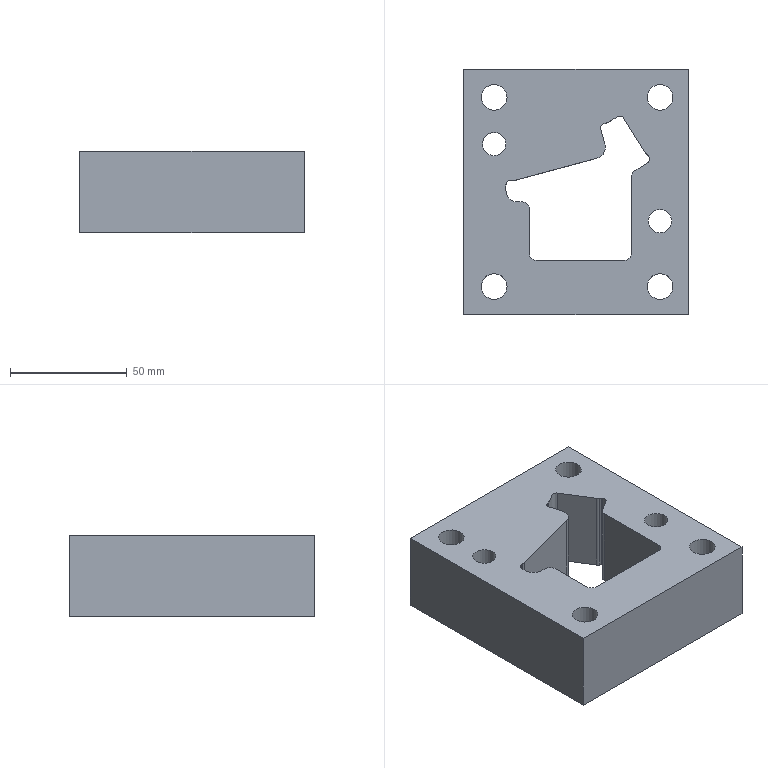Part | NX | features solid 2 | 1 solid | 52 faces | box 96 x 105 x 35 mm | volume 249889 mm3 | cylinder 27 | plane 24 | spline 1 | commonest cylinder face diameters 4 x8 11 x6 10 x5 6 x4 17 x4
STEP:
#1=CARTESIAN_POINT('',(298.719,63.299,43.));
#2=VERTEX_POINT('',#1);
#3=CARTESIAN_POINT('',(298.719,-41.701,43.));
#4=VERTEX_POINT('',#3);
#5=CARTESIAN_POINT('',(298.719,13.399,43.));
#6=DIRECTION('',(0.,-1.,0.));
#7=VECTOR('',#6,1000.);
#8=LINE('',#5,#7);
#9=EDGE_CURVE('',#2,#4,#8,.T.);
#10=ORIENTED_EDGE('',*,*,#9,.T.);
#11=CARTESIAN_POINT('',(298.719,-41.701,78.));
#12=VERTEX_POINT('',#11);
#13=CARTESIAN_POINT('',(298.719,-41.701,-28.));
#14=DIRECTION('',(0.,0.,1.));
#15=VECTOR('',#14,1000.);
#16=LINE('',#13,#15);
#17=EDGE_CURVE('',#4,#12,#16,.T.);
#18=ORIENTED_EDGE('',*,*,#17,.T.);
#19=CARTESIAN_POINT('',(298.719,63.299,78.));
#20=VERTEX_POINT('',#19);
#21=CARTESIAN_POINT('',(298.719,13.399,78.));
#22=DIRECTION('',(0.,-1.,0.));
#23=VECTOR('',#22,1000.);
#24=LINE('',#21,#23);
#25=EDGE_CURVE('',#12,#20,#24,.F.);
#26=ORIENTED_EDGE('',*,*,#25,.T.);
#27=CARTESIAN_POINT('',(298.719,63.299,-28.));
#28=DIRECTION('',(0.,0.,1.));
#29=VECTOR('',#28,1000.);
#30=LINE('',#27,#29);
#31=EDGE_CURVE('',#2,#20,#30,.T.);
#32=ORIENTED_EDGE('',*,*,#31,.F.);
#33=EDGE_LOOP('',(#10,#18,#26,#32));
#34=FACE_BOUND('',#33,.T.);
#35=CARTESIAN_POINT('',(298.719,13.399,-28.));
#36=DIRECTION('',(-1.,0.,0.));
#37=DIRECTION('',(0.,0.,1.));
#38=AXIS2_PLACEMENT_3D('',#35,#36,#37);
#39=PLANE('',#38);
#40=ADVANCED_FACE('',(#34),#39,.T.);
#41=CARTESIAN_POINT('',(394.719,63.299,78.));
#42=VERTEX_POINT('',#41);
#43=CARTESIAN_POINT('',(347.479,63.299,78.));
#44=DIRECTION('',(-1.,0.,0.));
#45=VECTOR('',#44,1000.);
#46=LINE('',#43,#45);
#47=EDGE_CURVE('',#20,#42,#46,.F.);
#48=ORIENTED_EDGE('',*,*,#47,.F.);
#49=ORIENTED_EDGE('',*,*,#25,.F.);
#50=CARTESIAN_POINT('',(394.719,-41.701,78.));
#51=VERTEX_POINT('',#50);
#52=CARTESIAN_POINT('',(347.479,-41.701,78.));
#53=DIRECTION('',(1.,0.,0.));
#54=VECTOR('',#53,1000.);
#55=LINE('',#52,#54);
#56=EDGE_CURVE('',#51,#12,#55,.F.);
#57=ORIENTED_EDGE('',*,*,#56,.F.);
#58=CARTESIAN_POINT('',(394.719,13.399,78.));
#59=DIRECTION('',(0.,1.,0.));
#60=VECTOR('',#59,1000.);
#61=LINE('',#58,#60);
#62=EDGE_CURVE('',#42,#51,#61,.F.);
#63=ORIENTED_EDGE('',*,*,#62,.F.);
#64=EDGE_LOOP('',(#48,#49,#57,#63));
#65=FACE_BOUND('',#64,.T.);
#66=CARTESIAN_POINT('',(387.719,-1.701,78.));
#67=VERTEX_POINT('',#66);
#68=CARTESIAN_POINT('',(382.719,-1.701,78.));
#69=DIRECTION('',(0.,0.,1.));
#70=DIRECTION('',(1.,0.,0.));
#71=AXIS2_PLACEMENT_3D('',#68,#69,#70);
#72=CIRCLE('',#71,5.);
#73=EDGE_CURVE('',#67,#67,#72,.T.);
#74=ORIENTED_EDGE('',*,*,#73,.F.);
#75=EDGE_LOOP('',(#74));
#76=FACE_BOUND('',#75,.T.);
#77=CARTESIAN_POINT('',(316.719,31.299,78.));
#78=VERTEX_POINT('',#77);
#79=CARTESIAN_POINT('',(311.719,31.299,78.));
#80=DIRECTION('',(0.,0.,1.));
#81=DIRECTION('',(1.,0.,0.));
#82=AXIS2_PLACEMENT_3D('',#79,#80,#81);
#83=CIRCLE('',#82,5.);
#84=EDGE_CURVE('',#78,#78,#83,.T.);
#85=ORIENTED_EDGE('',*,*,#84,.F.);
#86=EDGE_LOOP('',(#85));
#87=FACE_BOUND('',#86,.T.);
#88=CARTESIAN_POINT('',(317.219,51.299,78.));
#89=VERTEX_POINT('',#88);
#90=CARTESIAN_POINT('',(311.719,51.299,78.));
#91=DIRECTION('',(0.,0.,-1.));
#92=DIRECTION('',(1.,0.,0.));
#93=AXIS2_PLACEMENT_3D('',#90,#91,#92);
#94=CIRCLE('',#93,5.5);
#95=EDGE_CURVE('',#89,#89,#94,.T.);
#96=ORIENTED_EDGE('',*,*,#95,.T.);
#97=EDGE_LOOP('',(#96));
#98=FACE_BOUND('',#97,.T.);
#99=CARTESIAN_POINT('',(377.219,51.299,78.));
#100=VERTEX_POINT('',#99);
#101=CARTESIAN_POINT('',(382.719,51.299,78.));
#102=DIRECTION('',(0.,0.,1.));
#103=DIRECTION('',(-1.,0.,0.));
#104=AXIS2_PLACEMENT_3D('',#101,#102,#103);
#105=CIRCLE('',#104,5.5);
#106=EDGE_CURVE('',#100,#100,#105,.F.);
#107=ORIENTED_EDGE('',*,*,#106,.T.);
#108=EDGE_LOOP('',(#107));
#109=FACE_BOUND('',#108,.T.);
#110=CARTESIAN_POINT('',(377.219,-29.701,78.));
#111=VERTEX_POINT('',#110);
#112=CARTESIAN_POINT('',(382.719,-29.701,78.));
#113=DIRECTION('',(0.,0.,-1.));
#114=DIRECTION('',(-1.,0.,0.));
#115=AXIS2_PLACEMENT_3D('',#112,#113,#114);
#116=CIRCLE('',#115,5.5);
#117=EDGE_CURVE('',#111,#111,#116,.T.);
#118=ORIENTED_EDGE('',*,*,#117,.T.);
#119=EDGE_LOOP('',(#118));
#120=FACE_BOUND('',#119,.T.);
#121=CARTESIAN_POINT('',(317.219,-29.701,78.));
#122=VERTEX_POINT('',#121);
#123=CARTESIAN_POINT('',(311.719,-29.701,78.));
#124=DIRECTION('',(0.,0.,1.));
#125=DIRECTION('',(1.,0.,0.));
#126=AXIS2_PLACEMENT_3D('',#123,#124,#125);
#127=CIRCLE('',#126,5.5);
#128=EDGE_CURVE('',#122,#122,#127,.T.);
#129=ORIENTED_EDGE('',*,*,#128,.F.);
#130=EDGE_LOOP('',(#129));
#131=FACE_BOUND('',#130,.T.);
#132=CARTESIAN_POINT('',(321.719,6.5,78.));
#133=VERTEX_POINT('',#132);
#134=CARTESIAN_POINT('',(316.719,11.5,78.));
#135=VERTEX_POINT('',#134);
#136=CARTESIAN_POINT('',(321.719,11.5,78.));
#137=DIRECTION('',(0.,0.,-1.));
#138=DIRECTION('',(-1.,0.,0.));
#139=AXIS2_PLACEMENT_3D('',#136,#137,#138);
#140=CIRCLE('',#139,5.);
#141=EDGE_CURVE('',#133,#135,#140,.T.);
#142=ORIENTED_EDGE('',*,*,#141,.T.);
#143=CARTESIAN_POINT('',(316.719,13.767,78.));
#144=VERTEX_POINT('',#143);
#145=CARTESIAN_POINT('',(316.719,89.912,78.));
#146=DIRECTION('',(0.,1.,0.));
#147=VECTOR('',#146,1000.);
#148=LINE('',#145,#147);
#149=EDGE_CURVE('',#135,#144,#148,.T.);
#150=ORIENTED_EDGE('',*,*,#149,.T.);
#151=CARTESIAN_POINT('',(318.201,15.698,78.));
#152=VERTEX_POINT('',#151);
#153=CARTESIAN_POINT('',(318.719,13.767,78.));
#154=DIRECTION('',(0.,0.,-1.));
#155=DIRECTION('',(-1.,0.,0.));
#156=AXIS2_PLACEMENT_3D('',#153,#154,#155);
#157=CIRCLE('',#156,2.);
#158=EDGE_CURVE('',#144,#152,#157,.T.);
#159=ORIENTED_EDGE('',*,*,#158,.T.);
#160=CARTESIAN_POINT('',(318.626,15.812,78.));
#161=VERTEX_POINT('',#160);
#162=CARTESIAN_POINT('',(303.806,11.841,78.));
#163=DIRECTION('',(0.9659,0.2588,0.));
#164=VECTOR('',#163,1000.);
#165=LINE('',#162,#164);
#166=EDGE_CURVE('',#152,#161,#165,.T.);
#167=ORIENTED_EDGE('',*,*,#166,.T.);
#168=CARTESIAN_POINT('',(319.626,15.821,78.));
#169=VERTEX_POINT('',#168);
#170=CARTESIAN_POINT('',(319.143,13.88,78.));
#171=DIRECTION('',(0.,0.,-1.));
#172=DIRECTION('',(-1.,0.,0.));
#173=AXIS2_PLACEMENT_3D('',#170,#171,#172);
#174=CIRCLE('',#173,2.);
#175=EDGE_CURVE('',#161,#169,#174,.T.);
#176=ORIENTED_EDGE('',*,*,#175,.T.);
#177=CARTESIAN_POINT('',(320.626,15.831,78.));
#178=VERTEX_POINT('',#177);
#179=CARTESIAN_POINT('',(320.108,17.762,78.));
#180=DIRECTION('',(0.,0.,-1.));
#181=DIRECTION('',(-1.,0.,0.));
#182=AXIS2_PLACEMENT_3D('',#179,#180,#181);
#183=CIRCLE('',#182,2.);
#184=EDGE_CURVE('',#169,#178,#183,.F.);
#185=ORIENTED_EDGE('',*,*,#184,.T.);
#186=CARTESIAN_POINT('',(355.551,25.189,78.));
#187=VERTEX_POINT('',#186);
#188=CARTESIAN_POINT('',(320.626,15.831,78.));
#189=DIRECTION('',(0.9659,0.2588,0.));
#190=VECTOR('',#189,1000.);
#191=LINE('',#188,#190);
#192=EDGE_CURVE('',#178,#187,#191,.T.);
#193=ORIENTED_EDGE('',*,*,#192,.T.);
#194=CARTESIAN_POINT('',(359.061,31.404,78.));
#195=VERTEX_POINT('',#194);
#196=CARTESIAN_POINT('',(354.257,30.018,78.));
#197=DIRECTION('',(0.,0.,-1.));
#198=DIRECTION('',(-1.,0.,0.));
#199=AXIS2_PLACEMENT_3D('',#196,#197,#198);
#200=CIRCLE('',#199,5.);
#201=EDGE_CURVE('',#187,#195,#200,.F.);
#202=ORIENTED_EDGE('',*,*,#201,.T.);
#203=CARTESIAN_POINT('',(357.296,37.575,78.));
#204=VERTEX_POINT('',#203);
#205=CARTESIAN_POINT('',(359.061,31.404,78.));
#206=CARTESIAN_POINT('',(358.469,33.46,78.));
#207=CARTESIAN_POINT('',(357.879,35.516,78.));
#208=CARTESIAN_POINT('',(357.296,37.575,78.));
#209=B_SPLINE_CURVE_WITH_KNOTS('',3,(#205,#206,#207,#208),.UNSPECIFIED.,.F.,.F.,(4,4),(0.,0.006418),.UNSPECIFIED.);
#210=EDGE_CURVE('',#195,#204,#209,.T.);
#211=ORIENTED_EDGE('',*,*,#210,.T.);
#212=CARTESIAN_POINT('',(358.674,40.044,78.));
#213=VERTEX_POINT('',#212);
#214=CARTESIAN_POINT('',(359.22,38.12,78.));
#215=DIRECTION('',(0.,0.,-1.));
#216=DIRECTION('',(-1.,0.,0.));
#217=AXIS2_PLACEMENT_3D('',#214,#215,#216);
#218=CIRCLE('',#217,2.);
#219=EDGE_CURVE('',#213,#204,#218,.F.);
#220=ORIENTED_EDGE('',*,*,#219,.F.);
#221=CARTESIAN_POINT('',(359.771,40.356,78.));
#222=VERTEX_POINT('',#221);
#223=CARTESIAN_POINT('',(311.762,26.741,78.));
#224=DIRECTION('',(-0.9621,-0.2728,0.));
#225=VECTOR('',#224,1000.);
#226=LINE('',#223,#225);
#227=EDGE_CURVE('',#222,#213,#226,.T.);
#228=ORIENTED_EDGE('',*,*,#227,.F.);
#229=CARTESIAN_POINT('',(361.057,40.926,78.));
#230=VERTEX_POINT('',#229);
#231=CARTESIAN_POINT('',(358.407,45.166,78.));
#232=DIRECTION('',(0.,0.,-1.));
#233=DIRECTION('',(-1.,0.,0.));
#234=AXIS2_PLACEMENT_3D('',#231,#232,#233);
#235=CIRCLE('',#234,5.);
#236=EDGE_CURVE('',#230,#222,#235,.T.);
#237=ORIENTED_EDGE('',*,*,#236,.F.);
#238=CARTESIAN_POINT('',(364.368,42.995,78.));
#239=VERTEX_POINT('',#238);
#240=CARTESIAN_POINT('',(334.735,24.478,78.));
#241=DIRECTION('',(-0.848,-0.5299,0.));
#242=VECTOR('',#241,1000.);
#243=LINE('',#240,#242);
#244=EDGE_CURVE('',#239,#230,#243,.T.);
#245=ORIENTED_EDGE('',*,*,#244,.F.);
#246=CARTESIAN_POINT('',(367.124,42.358,78.));
#247=VERTEX_POINT('',#246);
#248=CARTESIAN_POINT('',(365.428,41.299,78.));
#249=DIRECTION('',(0.,0.,-1.));
#250=DIRECTION('',(-1.,0.,0.));
#251=AXIS2_PLACEMENT_3D('',#248,#249,#250);
#252=CIRCLE('',#251,2.);
#253=EDGE_CURVE('',#247,#239,#252,.F.);
#254=ORIENTED_EDGE('',*,*,#253,.F.);
#255=CARTESIAN_POINT('',(376.282,27.703,78.));
#256=VERTEX_POINT('',#255);
#257=CARTESIAN_POINT('',(367.124,42.358,78.));
#258=DIRECTION('',(0.5299,-0.848,0.));
#259=VECTOR('',#258,1000.);
#260=LINE('',#257,#259);
#261=EDGE_CURVE('',#247,#256,#260,.T.);
#262=ORIENTED_EDGE('',*,*,#261,.T.);
#263=CARTESIAN_POINT('',(377.007,27.014,78.));
#264=VERTEX_POINT('',#263);
#265=CARTESIAN_POINT('',(377.978,28.763,78.));
#266=DIRECTION('',(0.,0.,-1.));
#267=DIRECTION('',(-1.,0.,0.));
#268=AXIS2_PLACEMENT_3D('',#265,#266,#267);
#269=CIRCLE('',#268,2.);
#270=EDGE_CURVE('',#256,#264,#269,.F.);
#271=ORIENTED_EDGE('',*,*,#270,.T.);
#272=CARTESIAN_POINT('',(377.732,26.325,78.));
#273=VERTEX_POINT('',#272);
#274=CARTESIAN_POINT('',(376.036,25.266,78.));
#275=DIRECTION('',(0.,0.,-1.));
#276=DIRECTION('',(-1.,0.,0.));
#277=AXIS2_PLACEMENT_3D('',#274,#275,#276);
#278=CIRCLE('',#277,2.);
#279=EDGE_CURVE('',#264,#273,#278,.T.);
#280=ORIENTED_EDGE('',*,*,#279,.T.);
#281=CARTESIAN_POINT('',(377.937,25.998,78.));
#282=VERTEX_POINT('',#281);
#283=CARTESIAN_POINT('',(375.858,29.324,78.));
#284=DIRECTION('',(0.5299,-0.848,0.));
#285=VECTOR('',#284,1000.);
#286=LINE('',#283,#285);
#287=EDGE_CURVE('',#273,#282,#286,.T.);
#288=ORIENTED_EDGE('',*,*,#287,.T.);
#289=CARTESIAN_POINT('',(377.3,23.242,78.));
#290=VERTEX_POINT('',#289);
#291=CARTESIAN_POINT('',(376.24,24.938,78.));
#292=DIRECTION('',(0.,0.,-1.));
#293=DIRECTION('',(-1.,0.,0.));
#294=AXIS2_PLACEMENT_3D('',#291,#292,#293);
#295=CIRCLE('',#294,2.);
#296=EDGE_CURVE('',#282,#290,#295,.T.);
#297=ORIENTED_EDGE('',*,*,#296,.T.);
#298=CARTESIAN_POINT('',(371.926,19.884,78.));
#299=VERTEX_POINT('',#298);
#300=CARTESIAN_POINT('',(347.244,4.461,78.));
#301=DIRECTION('',(0.848,0.5299,0.));
#302=VECTOR('',#301,1000.);
#303=LINE('',#300,#302);
#304=EDGE_CURVE('',#299,#290,#303,.T.);
#305=ORIENTED_EDGE('',*,*,#304,.F.);
#306=CARTESIAN_POINT('',(370.516,17.34,78.));
#307=VERTEX_POINT('',#306);
#308=CARTESIAN_POINT('',(373.516,17.34,78.));
#309=DIRECTION('',(0.,0.,-1.));
#310=DIRECTION('',(-1.,0.,0.));
#311=AXIS2_PLACEMENT_3D('',#308,#309,#310);
#312=CIRCLE('',#311,3.);
#313=EDGE_CURVE('',#307,#299,#312,.T.);
#314=ORIENTED_EDGE('',*,*,#313,.F.);
#315=CARTESIAN_POINT('',(370.516,-15.5,78.));
#316=VERTEX_POINT('',#315);
#317=CARTESIAN_POINT('',(370.516,0.,78.));
#318=DIRECTION('',(0.,-1.,0.));
#319=VECTOR('',#318,1000.);
#320=LINE('',#317,#319);
#321=EDGE_CURVE('',#316,#307,#320,.F.);
#322=ORIENTED_EDGE('',*,*,#321,.F.);
#323=CARTESIAN_POINT('',(367.516,-18.5,78.));
#324=VERTEX_POINT('',#323);
#325=CARTESIAN_POINT('',(367.516,-15.5,78.));
#326=DIRECTION('',(0.,0.,-1.));
#327=DIRECTION('',(-1.,0.,0.));
#328=AXIS2_PLACEMENT_3D('',#325,#326,#327);
#329=CIRCLE('',#328,3.);
#330=EDGE_CURVE('',#316,#324,#329,.T.);
#331=ORIENTED_EDGE('',*,*,#330,.T.);
#332=CARTESIAN_POINT('',(329.719,-18.5,78.));
#333=VERTEX_POINT('',#332);
#334=CARTESIAN_POINT('',(297.,-18.5,78.));
#335=DIRECTION('',(1.,0.,0.));
#336=VECTOR('',#335,1000.);
#337=LINE('',#334,#336);
#338=EDGE_CURVE('',#333,#324,#337,.T.);
#339=ORIENTED_EDGE('',*,*,#338,.F.);
#340=CARTESIAN_POINT('',(326.719,-15.5,78.));
#341=VERTEX_POINT('',#340);
#342=CARTESIAN_POINT('',(329.719,-15.5,78.));
#343=DIRECTION('',(0.,0.,-1.));
#344=DIRECTION('',(-1.,0.,0.));
#345=AXIS2_PLACEMENT_3D('',#342,#343,#344);
#346=CIRCLE('',#345,3.);
#347=EDGE_CURVE('',#333,#341,#346,.T.);
#348=ORIENTED_EDGE('',*,*,#347,.T.);
#349=CARTESIAN_POINT('',(326.719,3.5,78.));
#350=VERTEX_POINT('',#349);
#351=CARTESIAN_POINT('',(326.719,6.5,78.));
#352=DIRECTION('',(0.,1.,0.));
#353=VECTOR('',#352,1000.);
#354=LINE('',#351,#353);
#355=EDGE_CURVE('',#341,#350,#354,.T.);
#356=ORIENTED_EDGE('',*,*,#355,.T.);
#357=CARTESIAN_POINT('',(323.719,6.5,78.));
#358=VERTEX_POINT('',#357);
#359=CARTESIAN_POINT('',(323.719,3.5,78.));
#360=DIRECTION('',(0.,0.,-1.));
#361=DIRECTION('',(-1.,0.,0.));
#362=AXIS2_PLACEMENT_3D('',#359,#360,#361);
#363=CIRCLE('',#362,3.);
#364=EDGE_CURVE('',#358,#350,#363,.T.);
#365=ORIENTED_EDGE('',*,*,#364,.F.);
#366=CARTESIAN_POINT('',(297.,6.5,78.));
#367=DIRECTION('',(1.,0.,0.));
#368=VECTOR('',#367,1000.);
#369=LINE('',#366,#368);
#370=EDGE_CURVE('',#133,#358,#369,.T.);
#371=ORIENTED_EDGE('',*,*,#370,.F.);
#372=EDGE_LOOP('',(#142,#150,#159,#167,#176,#185,#193,#202,#211,#220,#228,#237,#245,#254,#262,#271,#280,#288,#297,#305,#314,#322,#331,#339,#348,#356,#365,#371));
#373=FACE_BOUND('',#372,.T.);
#374=CARTESIAN_POINT('',(188.,0.,78.));
#375=DIRECTION('',(0.,0.,-1.));
#376=DIRECTION('',(-1.,0.,0.));
#377=AXIS2_PLACEMENT_3D('',#374,#375,#376);
#378=PLANE('',#377);
#379=ADVANCED_FACE('',(#65,#76,#87,#98,#109,#120,#131,#373),#378,.F.);
#380=CARTESIAN_POINT('',(394.719,-41.701,43.));
#381=VERTEX_POINT('',#380);
#382=CARTESIAN_POINT('',(347.479,-41.701,43.));
#383=DIRECTION('',(1.,0.,0.));
#384=VECTOR('',#383,1000.);
#385=LINE('',#382,#384);
#386=EDGE_CURVE('',#4,#381,#385,.T.);
#387=ORIENTED_EDGE('',*,*,#386,.F.);
#388=ORIENTED_EDGE('',*,*,#9,.F.);
#389=CARTESIAN_POINT('',(394.719,63.299,43.));
#390=VERTEX_POINT('',#389);
#391=CARTESIAN_POINT('',(347.479,63.299,43.));
#392=DIRECTION('',(-1.,0.,0.));
#393=VECTOR('',#392,1000.);
#394=LINE('',#391,#393);
#395=EDGE_CURVE('',#390,#2,#394,.T.);
#396=ORIENTED_EDGE('',*,*,#395,.F.);
#397=CARTESIAN_POINT('',(394.719,13.399,43.));
#398=DIRECTION('',(0.,1.,0.));
#399=VECTOR('',#398,1000.);
#400=LINE('',#397,#399);
#401=EDGE_CURVE('',#381,#390,#400,.T.);
#402=ORIENTED_EDGE('',*,*,#401,.F.);
#403=EDGE_LOOP('',(#387,#388,#396,#402));
#404=FACE_BOUND('',#403,.T.);
#405=CARTESIAN_POINT('',(320.219,-29.701,43.));
#406=VERTEX_POINT('',#405);
#407=CARTESIAN_POINT('',(311.719,-29.701,43.));
#408=DIRECTION('',(0.,0.,1.));
#409=DIRECTION('',(1.,0.,0.));
#410=AXIS2_PLACEMENT_3D('',#407,#408,#409);
#411=CIRCLE('',#410,8.5);
#412=EDGE_CURVE('',#406,#406,#411,.T.);
#413=ORIENTED_EDGE('',*,*,#412,.T.);
#414=EDGE_LOOP('',(#413));
#415=FACE_BOUND('',#414,.T.);
#416=CARTESIAN_POINT('',(374.219,-29.701,43.));
#417=VERTEX_POINT('',#416);
#418=CARTESIAN_POINT('',(382.719,-29.701,43.));
#419=DIRECTION('',(0.,0.,-1.));
#420=DIRECTION('',(-1.,0.,0.));
#421=AXIS2_PLACEMENT_3D('',#418,#419,#420);
#422=CIRCLE('',#421,8.5);
#423=EDGE_CURVE('',#417,#417,#422,.F.);
#424=ORIENTED_EDGE('',*,*,#423,.T.);
#425=EDGE_LOOP('',(#424));
#426=FACE_BOUND('',#425,.T.);
#427=CARTESIAN_POINT('',(374.219,51.299,43.));
#428=VERTEX_POINT('',#427);
#429=CARTESIAN_POINT('',(382.719,51.299,43.));
#430=DIRECTION('',(0.,0.,1.));
#431=DIRECTION('',(-1.,0.,0.));
#432=AXIS2_PLACEMENT_3D('',#429,#430,#431);
#433=CIRCLE('',#432,8.5);
#434=EDGE_CURVE('',#428,#428,#433,.T.);
#435=ORIENTED_EDGE('',*,*,#434,.T.);
#436=EDGE_LOOP('',(#435));
#437=FACE_BOUND('',#436,.T.);
#438=CARTESIAN_POINT('',(320.219,51.299,43.));
#439=VERTEX_POINT('',#438);
#440=CARTESIAN_POINT('',(311.719,51.299,43.));
#441=DIRECTION('',(0.,0.,-1.));
#442=DIRECTION('',(1.,0.,0.));
#443=AXIS2_PLACEMENT_3D('',#440,#441,#442);
#444=CIRCLE('',#443,8.5);
#445=EDGE_CURVE('',#439,#439,#444,.F.);
#446=ORIENTED_EDGE('',*,*,#445,.T.);
#447=EDGE_LOOP('',(#446));
#448=FACE_BOUND('',#447,.T.);
#449=CARTESIAN_POINT('',(317.219,31.299,43.));
#450=VERTEX_POINT('',#449);
#451=CARTESIAN_POINT('',(311.719,31.299,43.));
#452=DIRECTION('',(0.,0.,1.));
#453=DIRECTION('',(1.,0.,0.));
#454=AXIS2_PLACEMENT_3D('',#451,#452,#453);
#455=CIRCLE('',#454,5.5);
#456=EDGE_CURVE('',#450,#450,#455,.T.);
#457=ORIENTED_EDGE('',*,*,#456,.T.);
#458=EDGE_LOOP('',(#457));
#459=FACE_BOUND('',#458,.T.);
#460=CARTESIAN_POINT('',(388.219,-1.701,43.));
#461=VERTEX_POINT('',#460);
#462=CARTESIAN_POINT('',(382.719,-1.701,43.));
#463=DIRECTION('',(0.,0.,1.));
#464=DIRECTION('',(1.,0.,0.));
#465=AXIS2_PLACEMENT_3D('',#462,#463,#464);
#466=CIRCLE('',#465,5.5);
#467=EDGE_CURVE('',#461,#461,#466,.T.);
#468=ORIENTED_EDGE('',*,*,#467,.T.);
#469=EDGE_LOOP('',(#468));
#470=FACE_BOUND('',#469,.T.);
#471=CARTESIAN_POINT('',(318.201,15.698,43.));
#472=VERTEX_POINT('',#471);
#473=CARTESIAN_POINT('',(316.719,13.767,43.));
#474=VERTEX_POINT('',#473);
#475=CARTESIAN_POINT('',(318.719,13.767,43.));
#476=DIRECTION('',(0.,0.,-1.));
#477=DIRECTION('',(-1.,0.,0.));
#478=AXIS2_PLACEMENT_3D('',#475,#476,#477);
#479=CIRCLE('',#478,2.);
#480=EDGE_CURVE('',#472,#474,#479,.F.);
#481=ORIENTED_EDGE('',*,*,#480,.T.);
#482=CARTESIAN_POINT('',(316.719,11.5,43.));
#483=VERTEX_POINT('',#482);
#484=CARTESIAN_POINT('',(316.719,0.,43.));
#485=DIRECTION('',(0.,-1.,0.));
#486=VECTOR('',#485,1000.);
#487=LINE('',#484,#486);
#488=EDGE_CURVE('',#474,#483,#487,.T.);
#489=ORIENTED_EDGE('',*,*,#488,.T.);
#490=CARTESIAN_POINT('',(321.719,6.5,43.));
#491=VERTEX_POINT('',#490);
#492=CARTESIAN_POINT('',(321.719,11.5,43.));
#493=DIRECTION('',(0.,0.,-1.));
#494=DIRECTION('',(-1.,0.,0.));
#495=AXIS2_PLACEMENT_3D('',#492,#493,#494);
#496=CIRCLE('',#495,5.);
#497=EDGE_CURVE('',#483,#491,#496,.F.);
#498=ORIENTED_EDGE('',*,*,#497,.T.);
#499=CARTESIAN_POINT('',(323.719,6.5,43.));
#500=VERTEX_POINT('',#499);
#501=CARTESIAN_POINT('',(188.,6.5,43.));
#502=DIRECTION('',(-1.,0.,0.));
#503=VECTOR('',#502,1000.);
#504=LINE('',#501,#503);
#505=EDGE_CURVE('',#500,#491,#504,.T.);
#506=ORIENTED_EDGE('',*,*,#505,.F.);
#507=CARTESIAN_POINT('',(326.719,3.5,43.));
#508=VERTEX_POINT('',#507);
#509=CARTESIAN_POINT('',(323.719,3.5,43.));
#510=DIRECTION('',(0.,0.,-1.));
#511=DIRECTION('',(-1.,0.,0.));
#512=AXIS2_PLACEMENT_3D('',#509,#510,#511);
#513=CIRCLE('',#512,3.);
#514=EDGE_CURVE('',#500,#508,#513,.T.);
#515=ORIENTED_EDGE('',*,*,#514,.T.);
#516=CARTESIAN_POINT('',(326.719,-15.5,43.));
#517=VERTEX_POINT('',#516);
#518=CARTESIAN_POINT('',(326.719,0.,43.));
#519=DIRECTION('',(0.,-1.,0.));
#520=VECTOR('',#519,1000.);
#521=LINE('',#518,#520);
#522=EDGE_CURVE('',#508,#517,#521,.T.);
#523=ORIENTED_EDGE('',*,*,#522,.T.);
#524=CARTESIAN_POINT('',(329.719,-18.5,43.));
#525=VERTEX_POINT('',#524);
#526=CARTESIAN_POINT('',(329.719,-15.5,43.));
#527=DIRECTION('',(0.,0.,-1.));
#528=DIRECTION('',(-1.,0.,0.));
#529=AXIS2_PLACEMENT_3D('',#526,#527,#528);
#530=CIRCLE('',#529,3.);
#531=EDGE_CURVE('',#517,#525,#530,.F.);
#532=ORIENTED_EDGE('',*,*,#531,.T.);
#533=CARTESIAN_POINT('',(367.516,-18.5,43.));
#534=VERTEX_POINT('',#533);
#535=CARTESIAN_POINT('',(188.,-18.5,43.));
#536=DIRECTION('',(-1.,0.,0.));
#537=VECTOR('',#536,1000.);
#538=LINE('',#535,#537);
#539=EDGE_CURVE('',#534,#525,#538,.T.);
#540=ORIENTED_EDGE('',*,*,#539,.F.);
#541=CARTESIAN_POINT('',(370.516,-15.5,43.));
#542=VERTEX_POINT('',#541);
#543=CARTESIAN_POINT('',(367.516,-15.5,43.));
#544=DIRECTION('',(0.,0.,-1.));
#545=DIRECTION('',(-1.,0.,0.));
#546=AXIS2_PLACEMENT_3D('',#543,#544,#545);
#547=CIRCLE('',#546,3.);
#548=EDGE_CURVE('',#534,#542,#547,.F.);
#549=ORIENTED_EDGE('',*,*,#548,.T.);
#550=CARTESIAN_POINT('',(370.516,17.339,43.));
#551=VERTEX_POINT('',#550);
#552=CARTESIAN_POINT('',(370.516,0.,43.));
#553=DIRECTION('',(0.,-1.,0.));
#554=VECTOR('',#553,1000.);
#555=LINE('',#552,#554);
#556=EDGE_CURVE('',#542,#551,#555,.F.);
#557=ORIENTED_EDGE('',*,*,#556,.T.);
#558=CARTESIAN_POINT('',(371.926,19.884,43.));
#559=VERTEX_POINT('',#558);
#560=CARTESIAN_POINT('',(373.516,17.339,43.));
#561=DIRECTION('',(0.,0.,-1.));
#562=DIRECTION('',(-1.,0.,0.));
#563=AXIS2_PLACEMENT_3D('',#560,#561,#562);
#564=CIRCLE('',#563,3.);
#565=EDGE_CURVE('',#551,#559,#564,.T.);
#566=ORIENTED_EDGE('',*,*,#565,.T.);
#567=CARTESIAN_POINT('',(377.3,23.242,43.));
#568=VERTEX_POINT('',#567);
#569=CARTESIAN_POINT('',(230.713,-68.356,43.));
#570=DIRECTION('',(-0.848,-0.5299,0.));
#571=VECTOR('',#570,1000.);
#572=LINE('',#569,#571);
#573=EDGE_CURVE('',#568,#559,#572,.T.);
#574=ORIENTED_EDGE('',*,*,#573,.F.);
#575=CARTESIAN_POINT('',(377.936,25.998,43.));
#576=VERTEX_POINT('',#575);
#577=CARTESIAN_POINT('',(376.24,24.938,43.));
#578=DIRECTION('',(0.,0.,-1.));
#579=DIRECTION('',(-1.,0.,0.));
#580=AXIS2_PLACEMENT_3D('',#577,#578,#579);
#581=CIRCLE('',#580,2.);
#582=EDGE_CURVE('',#568,#576,#581,.F.);
#583=ORIENTED_EDGE('',*,*,#582,.T.);
#584=CARTESIAN_POINT('',(377.732,26.325,43.));
#585=VERTEX_POINT('',#584);
#586=CARTESIAN_POINT('',(336.283,92.657,43.));
#587=DIRECTION('',(-0.5299,0.848,0.));
#588=VECTOR('',#587,1000.);
#589=LINE('',#586,#588);
#590=EDGE_CURVE('',#576,#585,#589,.T.);
#591=ORIENTED_EDGE('',*,*,#590,.T.);
#592=CARTESIAN_POINT('',(377.007,27.014,43.));
#593=VERTEX_POINT('',#592);
#594=CARTESIAN_POINT('',(376.036,25.266,43.));
#595=DIRECTION('',(0.,0.,-1.));
#596=DIRECTION('',(-1.,0.,0.));
#597=AXIS2_PLACEMENT_3D('',#594,#595,#596);
#598=CIRCLE('',#597,2.);
#599=EDGE_CURVE('',#585,#593,#598,.F.);
#600=ORIENTED_EDGE('',*,*,#599,.T.);
#601=CARTESIAN_POINT('',(376.282,27.703,43.));
#602=VERTEX_POINT('',#601);
#603=CARTESIAN_POINT('',(377.978,28.762,43.));
#604=DIRECTION('',(0.,0.,-1.));
#605=DIRECTION('',(-1.,0.,0.));
#606=AXIS2_PLACEMENT_3D('',#603,#604,#605);
#607=CIRCLE('',#606,2.);
#608=EDGE_CURVE('',#593,#602,#607,.T.);
#609=ORIENTED_EDGE('',*,*,#608,.T.);
#610=CARTESIAN_POINT('',(367.124,42.358,43.));
#611=VERTEX_POINT('',#610);
#612=CARTESIAN_POINT('',(335.859,92.392,43.));
#613=DIRECTION('',(-0.5299,0.848,0.));
#614=VECTOR('',#613,1000.);
#615=LINE('',#612,#614);
#616=EDGE_CURVE('',#602,#611,#615,.T.);
#617=ORIENTED_EDGE('',*,*,#616,.T.);
#618=CARTESIAN_POINT('',(364.368,42.995,43.));
#619=VERTEX_POINT('',#618);
#620=CARTESIAN_POINT('',(365.428,41.299,43.));
#621=DIRECTION('',(0.,0.,-1.));
#622=DIRECTION('',(-1.,0.,0.));
#623=AXIS2_PLACEMENT_3D('',#620,#621,#622);
#624=CIRCLE('',#623,2.);
#625=EDGE_CURVE('',#619,#611,#624,.T.);
#626=ORIENTED_EDGE('',*,*,#625,.F.);
#627=CARTESIAN_POINT('',(361.057,40.926,43.));
#628=VERTEX_POINT('',#627);
#629=CARTESIAN_POINT('',(218.205,-48.338,43.));
#630=DIRECTION('',(0.848,0.5299,0.));
#631=VECTOR('',#630,1000.);
#632=LINE('',#629,#631);
#633=EDGE_CURVE('',#628,#619,#632,.T.);
#634=ORIENTED_EDGE('',*,*,#633,.F.);
#635=CARTESIAN_POINT('',(359.771,40.356,43.));
#636=VERTEX_POINT('',#635);
#637=CARTESIAN_POINT('',(358.407,45.166,43.));
#638=DIRECTION('',(0.,0.,-1.));
#639=DIRECTION('',(-1.,0.,0.));
#640=AXIS2_PLACEMENT_3D('',#637,#638,#639);
#641=CIRCLE('',#640,5.);
#642=EDGE_CURVE('',#628,#636,#641,.T.);
#643=ORIENTED_EDGE('',*,*,#642,.T.);
#644=CARTESIAN_POINT('',(358.674,40.044,43.));
#645=VERTEX_POINT('',#644);
#646=CARTESIAN_POINT('',(190.193,-7.734,43.));
#647=DIRECTION('',(0.9621,0.2728,0.));
#648=VECTOR('',#647,1000.);
#649=LINE('',#646,#648);
#650=EDGE_CURVE('',#645,#636,#649,.T.);
#651=ORIENTED_EDGE('',*,*,#650,.F.);
#652=CARTESIAN_POINT('',(357.296,37.575,43.));
#653=VERTEX_POINT('',#652);
#654=CARTESIAN_POINT('',(359.22,38.12,43.));
#655=DIRECTION('',(0.,0.,-1.));
#656=DIRECTION('',(-1.,0.,0.));
#657=AXIS2_PLACEMENT_3D('',#654,#655,#656);
#658=CIRCLE('',#657,2.);
#659=EDGE_CURVE('',#653,#645,#658,.T.);
#660=ORIENTED_EDGE('',*,*,#659,.F.);
#661=CARTESIAN_POINT('',(359.061,31.404,43.));
#662=VERTEX_POINT('',#661);
#663=CARTESIAN_POINT('',(357.296,37.575,43.));
#664=CARTESIAN_POINT('',(357.879,35.516,43.));
#665=CARTESIAN_POINT('',(358.468,33.46,43.));
#666=CARTESIAN_POINT('',(359.061,31.404,43.));
#667=B_SPLINE_CURVE_WITH_KNOTS('',3,(#663,#664,#665,#666),.UNSPECIFIED.,.F.,.F.,(4,4),(0.,0.006418),.UNSPECIFIED.);
#668=EDGE_CURVE('',#653,#662,#667,.T.);
#669=ORIENTED_EDGE('',*,*,#668,.T.);
#670=CARTESIAN_POINT('',(355.551,25.189,43.));
#671=VERTEX_POINT('',#670);
#672=CARTESIAN_POINT('',(354.257,30.018,43.));
#673=DIRECTION('',(0.,0.,-1.));
#674=DIRECTION('',(-1.,0.,0.));
#675=AXIS2_PLACEMENT_3D('',#672,#673,#674);
#676=CIRCLE('',#675,5.);
#677=EDGE_CURVE('',#662,#671,#676,.T.);
#678=ORIENTED_EDGE('',*,*,#677,.T.);
#679=CARTESIAN_POINT('',(320.626,15.831,43.));
#680=VERTEX_POINT('',#679);
#681=CARTESIAN_POINT('',(192.927,-18.386,43.));
#682=DIRECTION('',(-0.9659,-0.2588,0.));
#683=VECTOR('',#682,1000.);
#684=LINE('',#681,#683);
#685=EDGE_CURVE('',#671,#680,#684,.T.);
#686=ORIENTED_EDGE('',*,*,#685,.T.);
#687=CARTESIAN_POINT('',(319.626,15.821,43.));
#688=VERTEX_POINT('',#687);
#689=CARTESIAN_POINT('',(320.108,17.762,43.));
#690=DIRECTION('',(0.,0.,-1.));
#691=DIRECTION('',(-1.,0.,0.));
#692=AXIS2_PLACEMENT_3D('',#689,#690,#691);
#693=CIRCLE('',#692,2.);
#694=EDGE_CURVE('',#680,#688,#693,.T.);
#695=ORIENTED_EDGE('',*,*,#694,.T.);
#696=CARTESIAN_POINT('',(318.626,15.812,43.));
#697=VERTEX_POINT('',#696);
#698=CARTESIAN_POINT('',(319.143,13.88,43.));
#699=DIRECTION('',(0.,0.,-1.));
#700=DIRECTION('',(-1.,0.,0.));
#701=AXIS2_PLACEMENT_3D('',#698,#699,#700);
#702=CIRCLE('',#701,2.);
#703=EDGE_CURVE('',#688,#697,#702,.F.);
#704=ORIENTED_EDGE('',*,*,#703,.T.);
#705=CARTESIAN_POINT('',(192.797,-17.903,43.));
#706=DIRECTION('',(-0.9659,-0.2588,0.));
#707=VECTOR('',#706,1000.);
#708=LINE('',#705,#707);
#709=EDGE_CURVE('',#697,#472,#708,.T.);
#710=ORIENTED_EDGE('',*,*,#709,.T.);
#711=EDGE_LOOP('',(#481,#489,#498,#506,#515,#523,#532,#540,#549,#557,#566,#574,#583,#591,#600,#609,#617,#626,#634,#643,#651,#660,#669,#678,#686,#695,#704,#710));
#712=FACE_BOUND('',#711,.T.);
#713=CARTESIAN_POINT('',(188.,0.,43.));
#714=DIRECTION('',(0.,0.,-1.));
#715=DIRECTION('',(-1.,0.,0.));
#716=AXIS2_PLACEMENT_3D('',#713,#714,#715);
#717=PLANE('',#716);
#718=ADVANCED_FACE('',(#404,#415,#426,#437,#448,#459,#470,#712),#717,.T.);
#719=ORIENTED_EDGE('',*,*,#95,.F.);
#720=EDGE_LOOP('',(#719));
#721=FACE_BOUND('',#720,.T.);
#722=CARTESIAN_POINT('',(317.219,51.299,58.));
#723=VERTEX_POINT('',#722);
#724=CARTESIAN_POINT('',(311.719,51.299,58.));
#725=DIRECTION('',(0.,0.,-1.));
#726=DIRECTION('',(1.,0.,0.));
#727=AXIS2_PLACEMENT_3D('',#724,#725,#726);
#728=CIRCLE('',#727,5.5);
#729=EDGE_CURVE('',#723,#723,#728,.T.);
#730=ORIENTED_EDGE('',*,*,#729,.T.);
#731=EDGE_LOOP('',(#730));
#732=FACE_BOUND('',#731,.T.);
#733=CARTESIAN_POINT('',(311.719,51.299,78.));
#734=DIRECTION('',(0.,0.,1.));
#735=DIRECTION('',(1.,0.,0.));
#736=AXIS2_PLACEMENT_3D('',#733,#734,#735);
#737=CYLINDRICAL_SURFACE('',#736,5.5);
#738=ADVANCED_FACE('',(#721,#732),#737,.F.);
#739=ORIENTED_EDGE('',*,*,#729,.F.);
#740=EDGE_LOOP('',(#739));
#741=FACE_BOUND('',#740,.T.);
#742=CARTESIAN_POINT('',(320.219,51.299,58.));
#743=VERTEX_POINT('',#742);
#744=CARTESIAN_POINT('',(311.719,51.299,58.));
#745=DIRECTION('',(0.,0.,-1.));
#746=DIRECTION('',(1.,0.,0.));
#747=AXIS2_PLACEMENT_3D('',#744,#745,#746);
#748=CIRCLE('',#747,8.5);
#749=EDGE_CURVE('',#743,#743,#748,.T.);
#750=ORIENTED_EDGE('',*,*,#749,.T.);
#751=EDGE_LOOP('',(#750));
#752=FACE_BOUND('',#751,.T.);
#753=CARTESIAN_POINT('',(311.351,49.433,58.));
#754=DIRECTION('',(0.,0.,1.));
#755=DIRECTION('',(1.,0.,0.));
#756=AXIS2_PLACEMENT_3D('',#753,#754,#755);
#757=PLANE('',#756);
#758=ADVANCED_FACE('',(#741,#752),#757,.F.);
#759=ORIENTED_EDGE('',*,*,#749,.F.);
#760=EDGE_LOOP('',(#759));
#761=FACE_BOUND('',#760,.T.);
#762=ORIENTED_EDGE('',*,*,#445,.F.);
#763=EDGE_LOOP('',(#762));
#764=FACE_BOUND('',#763,.T.);
#765=CARTESIAN_POINT('',(311.719,51.299,43.));
#766=DIRECTION('',(0.,0.,1.));
#767=DIRECTION('',(1.,0.,0.));
#768=AXIS2_PLACEMENT_3D('',#765,#766,#767);
#769=CYLINDRICAL_SURFACE('',#768,8.5);
#770=ADVANCED_FACE('',(#761,#764),#769,.F.);
#771=CARTESIAN_POINT('',(374.219,51.299,58.));
#772=VERTEX_POINT('',#771);
#773=CARTESIAN_POINT('',(382.719,51.299,58.));
#774=DIRECTION('',(0.,0.,1.));
#775=DIRECTION('',(-1.,0.,0.));
#776=AXIS2_PLACEMENT_3D('',#773,#774,#775);
#777=CIRCLE('',#776,8.5);
#778=EDGE_CURVE('',#772,#772,#777,.F.);
#779=ORIENTED_EDGE('',*,*,#778,.F.);
#780=EDGE_LOOP('',(#779));
#781=FACE_BOUND('',#780,.T.);
#782=ORIENTED_EDGE('',*,*,#434,.F.);
#783=EDGE_LOOP('',(#782));
#784=FACE_BOUND('',#783,.T.);
#785=CARTESIAN_POINT('',(382.719,51.299,43.));
#786=DIRECTION('',(0.,0.,1.));
#787=DIRECTION('',(-1.,0.,0.));
#788=AXIS2_PLACEMENT_3D('',#785,#786,#787);
#789=CYLINDRICAL_SURFACE('',#788,8.5);
#790=ADVANCED_FACE('',(#781,#784),#789,.F.);
#791=CARTESIAN_POINT('',(377.219,51.299,58.));
#792=VERTEX_POINT('',#791);
#793=CARTESIAN_POINT('',(382.719,51.299,58.));
#794=DIRECTION('',(0.,0.,1.));
#795=DIRECTION('',(-1.,0.,0.));
#796=AXIS2_PLACEMENT_3D('',#793,#794,#795);
#797=CIRCLE('',#796,5.5);
#798=EDGE_CURVE('',#792,#792,#797,.F.);
#799=ORIENTED_EDGE('',*,*,#798,.F.);
#800=EDGE_LOOP('',(#799));
#801=FACE_BOUND('',#800,.T.);
#802=ORIENTED_EDGE('',*,*,#778,.T.);
#803=EDGE_LOOP('',(#802));
#804=FACE_BOUND('',#803,.T.);
#805=CARTESIAN_POINT('',(383.086,49.433,58.));
#806=DIRECTION('',(0.,0.,1.));
#807=DIRECTION('',(-1.,0.,0.));
#808=AXIS2_PLACEMENT_3D('',#805,#806,#807);
#809=PLANE('',#808);
#810=ADVANCED_FACE('',(#801,#804),#809,.F.);
#811=ORIENTED_EDGE('',*,*,#106,.F.);
#812=EDGE_LOOP('',(#811));
#813=FACE_BOUND('',#812,.T.);
#814=ORIENTED_EDGE('',*,*,#798,.T.);
#815=EDGE_LOOP('',(#814));
#816=FACE_BOUND('',#815,.T.);
#817=CARTESIAN_POINT('',(382.719,51.299,78.));
#818=DIRECTION('',(0.,0.,1.));
#819=DIRECTION('',(-1.,0.,0.));
#820=AXIS2_PLACEMENT_3D('',#817,#818,#819);
#821=CYLINDRICAL_SURFACE('',#820,5.5);
#822=ADVANCED_FACE('',(#813,#816),#821,.F.);
#823=CARTESIAN_POINT('',(317.219,-29.701,58.));
#824=VERTEX_POINT('',#823);
#825=CARTESIAN_POINT('',(311.719,-29.701,58.));
#826=DIRECTION('',(0.,0.,1.));
#827=DIRECTION('',(1.,0.,0.));
#828=AXIS2_PLACEMENT_3D('',#825,#826,#827);
#829=CIRCLE('',#828,5.5);
#830=EDGE_CURVE('',#824,#824,#829,.F.);
#831=ORIENTED_EDGE('',*,*,#830,.F.);
#832=EDGE_LOOP('',(#831));
#833=FACE_BOUND('',#832,.T.);
#834=CARTESIAN_POINT('',(320.219,-29.701,58.));
#835=VERTEX_POINT('',#834);
#836=CARTESIAN_POINT('',(311.719,-29.701,58.));
#837=DIRECTION('',(0.,0.,1.));
#838=DIRECTION('',(1.,0.,0.));
#839=AXIS2_PLACEMENT_3D('',#836,#837,#838);
#840=CIRCLE('',#839,8.5);
#841=EDGE_CURVE('',#835,#835,#840,.F.);
#842=ORIENTED_EDGE('',*,*,#841,.T.);
#843=EDGE_LOOP('',(#842));
#844=FACE_BOUND('',#843,.T.);
#845=CARTESIAN_POINT('',(311.351,-27.835,58.));
#846=DIRECTION('',(0.,0.,1.));
#847=DIRECTION('',(1.,0.,0.));
#848=AXIS2_PLACEMENT_3D('',#845,#846,#847);
#849=PLANE('',#848);
#850=ADVANCED_FACE('',(#833,#844),#849,.F.);
#851=CARTESIAN_POINT('',(377.219,-29.701,58.));
#852=VERTEX_POINT('',#851);
#853=CARTESIAN_POINT('',(382.719,-29.701,58.));
#854=DIRECTION('',(0.,0.,-1.));
#855=DIRECTION('',(-1.,0.,0.));
#856=AXIS2_PLACEMENT_3D('',#853,#854,#855);
#857=CIRCLE('',#856,5.5);
#858=EDGE_CURVE('',#852,#852,#857,.T.);
#859=ORIENTED_EDGE('',*,*,#858,.F.);
#860=EDGE_LOOP('',(#859));
#861=FACE_BOUND('',#860,.T.);
#862=CARTESIAN_POINT('',(374.219,-29.701,58.));
#863=VERTEX_POINT('',#862);
#864=CARTESIAN_POINT('',(382.719,-29.701,58.));
#865=DIRECTION('',(0.,0.,-1.));
#866=DIRECTION('',(-1.,0.,0.));
#867=AXIS2_PLACEMENT_3D('',#864,#865,#866);
#868=CIRCLE('',#867,8.5);
#869=EDGE_CURVE('',#863,#863,#868,.T.);
#870=ORIENTED_EDGE('',*,*,#869,.T.);
#871=EDGE_LOOP('',(#870));
#872=FACE_BOUND('',#871,.T.);
#873=CARTESIAN_POINT('',(383.086,-27.835,58.));
#874=DIRECTION('',(0.,0.,1.));
#875=DIRECTION('',(-1.,0.,0.));
#876=AXIS2_PLACEMENT_3D('',#873,#874,#875);
#877=PLANE('',#876);
#878=ADVANCED_FACE('',(#861,#872),#877,.F.);
#879=ORIENTED_EDGE('',*,*,#31,.T.);
#880=ORIENTED_EDGE('',*,*,#47,.T.);
#881=CARTESIAN_POINT('',(394.719,63.299,-28.));
#882=DIRECTION('',(0.,0.,1.));
#883=VECTOR('',#882,1000.);
#884=LINE('',#881,#883);
#885=EDGE_CURVE('',#390,#42,#884,.T.);
#886=ORIENTED_EDGE('',*,*,#885,.F.);
#887=ORIENTED_EDGE('',*,*,#395,.T.);
#888=EDGE_LOOP('',(#879,#880,#886,#887));
#889=FACE_BOUND('',#888,.T.);
#890=CARTESIAN_POINT('',(347.479,63.299,-28.));
#891=DIRECTION('',(0.,1.,0.));
#892=DIRECTION('',(0.,0.,1.));
#893=AXIS2_PLACEMENT_3D('',#890,#891,#892);
#894=PLANE('',#893);
#895=ADVANCED_FACE('',(#889),#894,.T.);
#896=ORIENTED_EDGE('',*,*,#401,.T.);
#897=ORIENTED_EDGE('',*,*,#885,.T.);
#898=ORIENTED_EDGE('',*,*,#62,.T.);
#899=CARTESIAN_POINT('',(394.719,-41.701,-28.));
#900=DIRECTION('',(0.,0.,1.));
#901=VECTOR('',#900,1000.);
#902=LINE('',#899,#901);
#903=EDGE_CURVE('',#381,#51,#902,.T.);
#904=ORIENTED_EDGE('',*,*,#903,.F.);
#905=EDGE_LOOP('',(#896,#897,#898,#904));
#906=FACE_BOUND('',#905,.T.);
#907=CARTESIAN_POINT('',(394.719,13.399,-28.));
#908=DIRECTION('',(1.,0.,0.));
#909=DIRECTION('',(0.,0.,-1.));
#910=AXIS2_PLACEMENT_3D('',#907,#908,#909);
#911=PLANE('',#910);
#912=ADVANCED_FACE('',(#906),#911,.T.);
#913=ORIENTED_EDGE('',*,*,#903,.T.);
#914=ORIENTED_EDGE('',*,*,#56,.T.);
#915=ORIENTED_EDGE('',*,*,#17,.F.);
#916=ORIENTED_EDGE('',*,*,#386,.T.);
#917=EDGE_LOOP('',(#913,#914,#915,#916));
#918=FACE_BOUND('',#917,.T.);
#919=CARTESIAN_POINT('',(347.479,-41.701,-28.));
#920=DIRECTION('',(0.,-1.,0.));
#921=DIRECTION('',(0.,0.,-1.));
#922=AXIS2_PLACEMENT_3D('',#919,#920,#921);
#923=PLANE('',#922);
#924=ADVANCED_FACE('',(#918),#923,.T.);
#925=ORIENTED_EDGE('',*,*,#128,.T.);
#926=EDGE_LOOP('',(#925));
#927=FACE_BOUND('',#926,.T.);
#928=ORIENTED_EDGE('',*,*,#830,.T.);
#929=EDGE_LOOP('',(#928));
#930=FACE_BOUND('',#929,.T.);
#931=CARTESIAN_POINT('',(311.719,-29.701,78.));
#932=DIRECTION('',(0.,0.,1.));
#933=DIRECTION('',(1.,0.,0.));
#934=AXIS2_PLACEMENT_3D('',#931,#932,#933);
#935=CYLINDRICAL_SURFACE('',#934,5.5);
#936=ADVANCED_FACE('',(#927,#930),#935,.F.);
#937=ORIENTED_EDGE('',*,*,#117,.F.);
#938=EDGE_LOOP('',(#937));
#939=FACE_BOUND('',#938,.T.);
#940=ORIENTED_EDGE('',*,*,#858,.T.);
#941=EDGE_LOOP('',(#940));
#942=FACE_BOUND('',#941,.T.);
#943=CARTESIAN_POINT('',(382.719,-29.701,78.));
#944=DIRECTION('',(0.,0.,1.));
#945=DIRECTION('',(-1.,0.,0.));
#946=AXIS2_PLACEMENT_3D('',#943,#944,#945);
#947=CYLINDRICAL_SURFACE('',#946,5.5);
#948=ADVANCED_FACE('',(#939,#942),#947,.F.);
#949=ORIENTED_EDGE('',*,*,#841,.F.);
#950=EDGE_LOOP('',(#949));
#951=FACE_BOUND('',#950,.T.);
#952=ORIENTED_EDGE('',*,*,#412,.F.);
#953=EDGE_LOOP('',(#952));
#954=FACE_BOUND('',#953,.T.);
#955=CARTESIAN_POINT('',(311.719,-29.701,43.));
#956=DIRECTION('',(0.,0.,1.));
#957=DIRECTION('',(1.,0.,0.));
#958=AXIS2_PLACEMENT_3D('',#955,#956,#957);
#959=CYLINDRICAL_SURFACE('',#958,8.5);
#960=ADVANCED_FACE('',(#951,#954),#959,.F.);
#961=ORIENTED_EDGE('',*,*,#869,.F.);
#962=EDGE_LOOP('',(#961));
#963=FACE_BOUND('',#962,.T.);
#964=ORIENTED_EDGE('',*,*,#423,.F.);
#965=EDGE_LOOP('',(#964));
#966=FACE_BOUND('',#965,.T.);
#967=CARTESIAN_POINT('',(382.719,-29.701,43.));
#968=DIRECTION('',(0.,0.,1.));
#969=DIRECTION('',(-1.,0.,0.));
#970=AXIS2_PLACEMENT_3D('',#967,#968,#969);
#971=CYLINDRICAL_SURFACE('',#970,8.5);
#972=ADVANCED_FACE('',(#963,#966),#971,.F.);
#973=ORIENTED_EDGE('',*,*,#84,.T.);
#974=EDGE_LOOP('',(#973));
#975=FACE_BOUND('',#974,.T.);
#976=CARTESIAN_POINT('',(316.719,31.299,58.));
#977=VERTEX_POINT('',#976);
#978=CARTESIAN_POINT('',(311.719,31.299,58.));
#979=DIRECTION('',(0.,0.,1.));
#980=DIRECTION('',(1.,0.,0.));
#981=AXIS2_PLACEMENT_3D('',#978,#979,#980);
#982=CIRCLE('',#981,5.);
#983=EDGE_CURVE('',#977,#977,#982,.F.);
#984=ORIENTED_EDGE('',*,*,#983,.T.);
#985=EDGE_LOOP('',(#984));
#986=FACE_BOUND('',#985,.T.);
#987=CARTESIAN_POINT('',(311.719,31.299,78.));
#988=DIRECTION('',(0.,0.,1.));
#989=DIRECTION('',(1.,0.,0.));
#990=AXIS2_PLACEMENT_3D('',#987,#988,#989);
#991=CYLINDRICAL_SURFACE('',#990,5.);
#992=ADVANCED_FACE('',(#975,#986),#991,.F.);
#993=ORIENTED_EDGE('',*,*,#983,.F.);
#994=EDGE_LOOP('',(#993));
#995=FACE_BOUND('',#994,.T.);
#996=CARTESIAN_POINT('',(317.219,31.299,58.));
#997=VERTEX_POINT('',#996);
#998=CARTESIAN_POINT('',(311.719,31.299,58.));
#999=DIRECTION('',(0.,0.,1.));
#1000=DIRECTION('',(1.,0.,0.));
#1001=AXIS2_PLACEMENT_3D('',#998,#999,#1000);
#1002=CIRCLE('',#1001,5.5);
#1003=EDGE_CURVE('',#997,#997,#1002,.F.);
#1004=ORIENTED_EDGE('',*,*,#1003,.T.);
#1005=EDGE_LOOP('',(#1004));
#1006=FACE_BOUND('',#1005,.T.);
#1007=CARTESIAN_POINT('',(312.444,30.227,58.));
#1008=DIRECTION('',(0.,0.,1.));
#1009=DIRECTION('',(1.,0.,0.));
#1010=AXIS2_PLACEMENT_3D('',#1007,#1008,#1009);
#1011=PLANE('',#1010);
#1012=ADVANCED_FACE('',(#995,#1006),#1011,.F.);
#1013=ORIENTED_EDGE('',*,*,#1003,.F.);
#1014=EDGE_LOOP('',(#1013));
#1015=FACE_BOUND('',#1014,.T.);
#1016=ORIENTED_EDGE('',*,*,#456,.F.);
#1017=EDGE_LOOP('',(#1016));
#1018=FACE_BOUND('',#1017,.T.);
#1019=CARTESIAN_POINT('',(311.719,31.299,43.));
#1020=DIRECTION('',(0.,0.,1.));
#1021=DIRECTION('',(1.,0.,0.));
#1022=AXIS2_PLACEMENT_3D('',#1019,#1020,#1021);
#1023=CYLINDRICAL_SURFACE('',#1022,5.5);
#1024=ADVANCED_FACE('',(#1015,#1018),#1023,.F.);
#1025=ORIENTED_EDGE('',*,*,#73,.T.);
#1026=EDGE_LOOP('',(#1025));
#1027=FACE_BOUND('',#1026,.T.);
#1028=CARTESIAN_POINT('',(387.719,-1.701,58.));
#1029=VERTEX_POINT('',#1028);
#1030=CARTESIAN_POINT('',(382.719,-1.701,58.));
#1031=DIRECTION('',(0.,0.,1.));
#1032=DIRECTION('',(1.,0.,0.));
#1033=AXIS2_PLACEMENT_3D('',#1030,#1031,#1032);
#1034=CIRCLE('',#1033,5.);
#1035=EDGE_CURVE('',#1029,#1029,#1034,.F.);
#1036=ORIENTED_EDGE('',*,*,#1035,.T.);
#1037=EDGE_LOOP('',(#1036));
#1038=FACE_BOUND('',#1037,.T.);
#1039=CARTESIAN_POINT('',(382.719,-1.701,78.));
#1040=DIRECTION('',(0.,0.,1.));
#1041=DIRECTION('',(1.,0.,0.));
#1042=AXIS2_PLACEMENT_3D('',#1039,#1040,#1041);
#1043=CYLINDRICAL_SURFACE('',#1042,5.);
#1044=ADVANCED_FACE('',(#1027,#1038),#1043,.F.);
#1045=ORIENTED_EDGE('',*,*,#1035,.F.);
#1046=EDGE_LOOP('',(#1045));
#1047=FACE_BOUND('',#1046,.T.);
#1048=CARTESIAN_POINT('',(388.219,-1.701,58.));
#1049=VERTEX_POINT('',#1048);
#1050=CARTESIAN_POINT('',(382.719,-1.701,58.));
#1051=DIRECTION('',(0.,0.,1.));
#1052=DIRECTION('',(1.,0.,0.));
#1053=AXIS2_PLACEMENT_3D('',#1050,#1051,#1052);
#1054=CIRCLE('',#1053,5.5);
#1055=EDGE_CURVE('',#1049,#1049,#1054,.F.);
#1056=ORIENTED_EDGE('',*,*,#1055,.T.);
#1057=EDGE_LOOP('',(#1056));
#1058=FACE_BOUND('',#1057,.T.);
#1059=CARTESIAN_POINT('',(382.126,-0.6285,58.));
#1060=DIRECTION('',(0.,0.,1.));
#1061=DIRECTION('',(1.,0.,0.));
#1062=AXIS2_PLACEMENT_3D('',#1059,#1060,#1061);
#1063=PLANE('',#1062);
#1064=ADVANCED_FACE('',(#1047,#1058),#1063,.F.);
#1065=ORIENTED_EDGE('',*,*,#1055,.F.);
#1066=EDGE_LOOP('',(#1065));
#1067=FACE_BOUND('',#1066,.T.);
#1068=ORIENTED_EDGE('',*,*,#467,.F.);
#1069=EDGE_LOOP('',(#1068));
#1070=FACE_BOUND('',#1069,.T.);
#1071=CARTESIAN_POINT('',(382.719,-1.701,43.));
#1072=DIRECTION('',(0.,0.,1.));
#1073=DIRECTION('',(1.,0.,0.));
#1074=AXIS2_PLACEMENT_3D('',#1071,#1072,#1073);
#1075=CYLINDRICAL_SURFACE('',#1074,5.5);
#1076=ADVANCED_FACE('',(#1067,#1070),#1075,.F.);
#1077=ORIENTED_EDGE('',*,*,#573,.T.);
#1078=CARTESIAN_POINT('',(371.926,19.884,-8.));
#1079=DIRECTION('',(-0.000000369,-0.000000231,-1.));
#1080=VECTOR('',#1079,1000.);
#1081=LINE('',#1078,#1080);
#1082=EDGE_CURVE('',#559,#299,#1081,.F.);
#1083=ORIENTED_EDGE('',*,*,#1082,.T.);
#1084=ORIENTED_EDGE('',*,*,#304,.T.);
#1085=CARTESIAN_POINT('',(377.3,23.242,-8.));
#1086=DIRECTION('',(0.000000369,0.000000231,1.));
#1087=VECTOR('',#1086,1000.);
#1088=LINE('',#1085,#1087);
#1089=EDGE_CURVE('',#290,#568,#1088,.F.);
#1090=ORIENTED_EDGE('',*,*,#1089,.T.);
#1091=EDGE_LOOP('',(#1077,#1083,#1084,#1090));
#1092=FACE_BOUND('',#1091,.T.);
#1093=CARTESIAN_POINT('',(347.244,4.461,-8.));
#1094=DIRECTION('',(0.5299,-0.848,0.));
#1095=DIRECTION('',(0.848,0.5299,0.));
#1096=AXIS2_PLACEMENT_3D('',#1093,#1094,#1095);
#1097=PLANE('',#1096);
#1098=ADVANCED_FACE('',(#1092),#1097,.F.);
#1099=ORIENTED_EDGE('',*,*,#556,.F.);
#1100=CARTESIAN_POINT('',(370.516,-15.5,19.));
#1101=DIRECTION('',(0.000000369,0.000000231,1.));
#1102=VECTOR('',#1101,1000.);
#1103=LINE('',#1100,#1102);
#1104=EDGE_CURVE('',#542,#316,#1103,.T.);
#1105=ORIENTED_EDGE('',*,*,#1104,.T.);
#1106=ORIENTED_EDGE('',*,*,#321,.T.);
#1107=CARTESIAN_POINT('',(370.516,17.339,19.));
#1108=DIRECTION('',(0.000000369,0.000000231,1.));
#1109=VECTOR('',#1108,1000.);
#1110=LINE('',#1107,#1109);
#1111=EDGE_CURVE('',#307,#551,#1110,.F.);
#1112=ORIENTED_EDGE('',*,*,#1111,.T.);
#1113=EDGE_LOOP('',(#1099,#1105,#1106,#1112));
#1114=FACE_BOUND('',#1113,.T.);
#1115=CARTESIAN_POINT('',(370.516,119.002,19.));
#1116=DIRECTION('',(1.,0.,-0.000000369));
#1117=DIRECTION('',(-0.000000369,0.,-1.));
#1118=AXIS2_PLACEMENT_3D('',#1115,#1116,#1117);
#1119=PLANE('',#1118);
#1120=ADVANCED_FACE('',(#1114),#1119,.F.);
#1121=ORIENTED_EDGE('',*,*,#539,.T.);
#1122=CARTESIAN_POINT('',(329.719,-18.5,-8.));
#1123=DIRECTION('',(0.000000369,0.000000231,1.));
#1124=VECTOR('',#1123,1000.);
#1125=LINE('',#1122,#1124);
#1126=EDGE_CURVE('',#525,#333,#1125,.T.);
#1127=ORIENTED_EDGE('',*,*,#1126,.T.);
#1128=ORIENTED_EDGE('',*,*,#338,.T.);
#1129=CARTESIAN_POINT('',(367.516,-18.5,-8.));
#1130=DIRECTION('',(-0.000000369,-0.000000231,-1.));
#1131=VECTOR('',#1130,1000.);
#1132=LINE('',#1129,#1131);
#1133=EDGE_CURVE('',#324,#534,#1132,.T.);
#1134=ORIENTED_EDGE('',*,*,#1133,.T.);
#1135=EDGE_LOOP('',(#1121,#1127,#1128,#1134));
#1136=FACE_BOUND('',#1135,.T.);
#1137=CARTESIAN_POINT('',(297.,-18.5,-8.));
#1138=DIRECTION('',(0.,-1.,0.000000231));
#1139=DIRECTION('',(0.,-0.000000231,-1.));
#1140=AXIS2_PLACEMENT_3D('',#1137,#1138,#1139);
#1141=PLANE('',#1140);
#1142=ADVANCED_FACE('',(#1136),#1141,.F.);
#1143=ORIENTED_EDGE('',*,*,#355,.F.);
#1144=CARTESIAN_POINT('',(326.719,-15.5,-8.));
#1145=DIRECTION('',(0.000000369,0.000000231,1.));
#1146=VECTOR('',#1145,1000.);
#1147=LINE('',#1144,#1146);
#1148=EDGE_CURVE('',#341,#517,#1147,.F.);
#1149=ORIENTED_EDGE('',*,*,#1148,.T.);
#1150=ORIENTED_EDGE('',*,*,#522,.F.);
#1151=CARTESIAN_POINT('',(326.719,3.5,-8.));
#1152=DIRECTION('',(0.000000369,0.000000231,1.));
#1153=VECTOR('',#1152,1000.);
#1154=LINE('',#1151,#1153);
#1155=EDGE_CURVE('',#508,#350,#1154,.T.);
#1156=ORIENTED_EDGE('',*,*,#1155,.T.);
#1157=EDGE_LOOP('',(#1143,#1149,#1150,#1156));
#1158=FACE_BOUND('',#1157,.T.);
#1159=CARTESIAN_POINT('',(326.719,6.5,-8.));
#1160=DIRECTION('',(1.,0.,-0.000000369));
#1161=DIRECTION('',(0.000000369,0.000000231,1.));
#1162=AXIS2_PLACEMENT_3D('',#1159,#1160,#1161);
#1163=PLANE('',#1162);
#1164=ADVANCED_FACE('',(#1158),#1163,.T.);
#1165=CARTESIAN_POINT('',(323.719,6.5,-8.));
#1166=DIRECTION('',(0.000000369,0.000000231,1.));
#1167=VECTOR('',#1166,1000.);
#1168=LINE('',#1165,#1167);
#1169=EDGE_CURVE('',#358,#500,#1168,.F.);
#1170=ORIENTED_EDGE('',*,*,#1169,.F.);
#1171=ORIENTED_EDGE('',*,*,#364,.T.);
#1172=ORIENTED_EDGE('',*,*,#1155,.F.);
#1173=ORIENTED_EDGE('',*,*,#514,.F.);
#1174=EDGE_LOOP('',(#1170,#1171,#1172,#1173));
#1175=FACE_BOUND('',#1174,.T.);
#1176=CARTESIAN_POINT('',(323.719,3.5,-8.));
#1177=DIRECTION('',(0.000000369,0.000000231,1.));
#1178=DIRECTION('',(1.,0.,-0.000000369));
#1179=AXIS2_PLACEMENT_3D('',#1176,#1177,#1178);
#1180=CYLINDRICAL_SURFACE('',#1179,3.);
#1181=ADVANCED_FACE('',(#1175),#1180,.T.);
#1182=ORIENTED_EDGE('',*,*,#505,.T.);
#1183=CARTESIAN_POINT('',(321.719,6.5,-8.));
#1184=DIRECTION('',(0.000000369,0.000000231,1.));
#1185=VECTOR('',#1184,1000.);
#1186=LINE('',#1183,#1185);
#1187=EDGE_CURVE('',#133,#491,#1186,.F.);
#1188=ORIENTED_EDGE('',*,*,#1187,.F.);
#1189=ORIENTED_EDGE('',*,*,#370,.T.);
#1190=ORIENTED_EDGE('',*,*,#1169,.T.);
#1191=EDGE_LOOP('',(#1182,#1188,#1189,#1190));
#1192=FACE_BOUND('',#1191,.T.);
#1193=CARTESIAN_POINT('',(297.,6.5,-8.));
#1194=DIRECTION('',(0.,-1.,0.000000231));
#1195=DIRECTION('',(0.,-0.000000231,-1.));
#1196=AXIS2_PLACEMENT_3D('',#1193,#1194,#1195);
#1197=PLANE('',#1196);
#1198=ADVANCED_FACE('',(#1192),#1197,.F.);
#1199=ORIENTED_EDGE('',*,*,#1111,.F.);
#1200=ORIENTED_EDGE('',*,*,#313,.T.);
#1201=ORIENTED_EDGE('',*,*,#1082,.F.);
#1202=ORIENTED_EDGE('',*,*,#565,.F.);
#1203=EDGE_LOOP('',(#1199,#1200,#1201,#1202));
#1204=FACE_BOUND('',#1203,.T.);
#1205=CARTESIAN_POINT('',(373.516,17.339,19.));
#1206=DIRECTION('',(-0.000000369,-0.000000231,-1.));
#1207=DIRECTION('',(-1.,0.,0.000000369));
#1208=AXIS2_PLACEMENT_3D('',#1205,#1206,#1207);
#1209=CYLINDRICAL_SURFACE('',#1208,3.);
#1210=ADVANCED_FACE('',(#1204),#1209,.T.);
#1211=ORIENTED_EDGE('',*,*,#1089,.F.);
#1212=ORIENTED_EDGE('',*,*,#296,.F.);
#1213=CARTESIAN_POINT('',(377.936,25.998,-8.));
#1214=DIRECTION('',(0.000000369,0.000000231,1.));
#1215=VECTOR('',#1214,1000.);
#1216=LINE('',#1213,#1215);
#1217=EDGE_CURVE('',#282,#576,#1216,.F.);
#1218=ORIENTED_EDGE('',*,*,#1217,.T.);
#1219=ORIENTED_EDGE('',*,*,#582,.F.);
#1220=EDGE_LOOP('',(#1211,#1212,#1218,#1219));
#1221=FACE_BOUND('',#1220,.T.);
#1222=CARTESIAN_POINT('',(376.24,24.938,-8.));
#1223=DIRECTION('',(0.000000369,0.000000231,1.));
#1224=DIRECTION('',(1.,0.,-0.000000369));
#1225=AXIS2_PLACEMENT_3D('',#1222,#1223,#1224);
#1226=CYLINDRICAL_SURFACE('',#1225,2.);
#1227=ADVANCED_FACE('',(#1221),#1226,.F.);
#1228=ORIENTED_EDGE('',*,*,#1217,.F.);
#1229=ORIENTED_EDGE('',*,*,#287,.F.);
#1230=CARTESIAN_POINT('',(377.732,26.325,-8.));
#1231=DIRECTION('',(0.000000369,0.000000231,1.));
#1232=VECTOR('',#1231,1000.);
#1233=LINE('',#1230,#1232);
#1234=EDGE_CURVE('',#273,#585,#1233,.F.);
#1235=ORIENTED_EDGE('',*,*,#1234,.T.);
#1236=ORIENTED_EDGE('',*,*,#590,.F.);
#1237=EDGE_LOOP('',(#1228,#1229,#1235,#1236));
#1238=FACE_BOUND('',#1237,.T.);
#1239=CARTESIAN_POINT('',(375.858,29.324,-8.));
#1240=DIRECTION('',(-0.848,-0.5299,0.000000435));
#1241=DIRECTION('',(0.5299,-0.848,0.));
#1242=AXIS2_PLACEMENT_3D('',#1239,#1240,#1241);
#1243=PLANE('',#1242);
#1244=ADVANCED_FACE('',(#1238),#1243,.T.);
#1245=ORIENTED_EDGE('',*,*,#1234,.F.);
#1246=ORIENTED_EDGE('',*,*,#279,.F.);
#1247=CARTESIAN_POINT('',(377.007,27.014,-8.));
#1248=DIRECTION('',(0.000000369,0.000000231,1.));
#1249=VECTOR('',#1248,1000.);
#1250=LINE('',#1247,#1249);
#1251=EDGE_CURVE('',#264,#593,#1250,.F.);
#1252=ORIENTED_EDGE('',*,*,#1251,.T.);
#1253=ORIENTED_EDGE('',*,*,#599,.F.);
#1254=EDGE_LOOP('',(#1245,#1246,#1252,#1253));
#1255=FACE_BOUND('',#1254,.T.);
#1256=CARTESIAN_POINT('',(376.036,25.266,-8.));
#1257=DIRECTION('',(0.000000369,0.000000231,1.));
#1258=DIRECTION('',(1.,0.,-0.000000369));
#1259=AXIS2_PLACEMENT_3D('',#1256,#1257,#1258);
#1260=CYLINDRICAL_SURFACE('',#1259,2.);
#1261=ADVANCED_FACE('',(#1255),#1260,.F.);
#1262=ORIENTED_EDGE('',*,*,#1251,.F.);
#1263=ORIENTED_EDGE('',*,*,#270,.F.);
#1264=CARTESIAN_POINT('',(376.282,27.703,-8.));
#1265=DIRECTION('',(0.000000369,0.000000231,1.));
#1266=VECTOR('',#1265,1000.);
#1267=LINE('',#1264,#1266);
#1268=EDGE_CURVE('',#256,#602,#1267,.F.);
#1269=ORIENTED_EDGE('',*,*,#1268,.T.);
#1270=ORIENTED_EDGE('',*,*,#608,.F.);
#1271=EDGE_LOOP('',(#1262,#1263,#1269,#1270));
#1272=FACE_BOUND('',#1271,.T.);
#1273=CARTESIAN_POINT('',(377.978,28.762,-8.));
#1274=DIRECTION('',(0.000000369,0.000000231,1.));
#1275=DIRECTION('',(1.,0.,-0.000000369));
#1276=AXIS2_PLACEMENT_3D('',#1273,#1274,#1275);
#1277=CYLINDRICAL_SURFACE('',#1276,2.);
#1278=ADVANCED_FACE('',(#1272),#1277,.T.);
#1279=ORIENTED_EDGE('',*,*,#1268,.F.);
#1280=ORIENTED_EDGE('',*,*,#261,.F.);
#1281=CARTESIAN_POINT('',(367.124,42.358,82.));
#1282=DIRECTION('',(-0.000000369,-0.000000231,-1.));
#1283=VECTOR('',#1282,1000.);
#1284=LINE('',#1281,#1283);
#1285=EDGE_CURVE('',#247,#611,#1284,.T.);
#1286=ORIENTED_EDGE('',*,*,#1285,.T.);
#1287=ORIENTED_EDGE('',*,*,#616,.F.);
#1288=EDGE_LOOP('',(#1279,#1280,#1286,#1287));
#1289=FACE_BOUND('',#1288,.T.);
#1290=CARTESIAN_POINT('',(367.124,42.358,-8.));
#1291=DIRECTION('',(-0.848,-0.5299,0.000000435));
#1292=DIRECTION('',(0.5299,-0.848,0.));
#1293=AXIS2_PLACEMENT_3D('',#1290,#1291,#1292);
#1294=PLANE('',#1293);
#1295=ADVANCED_FACE('',(#1289),#1294,.T.);
#1296=ORIENTED_EDGE('',*,*,#625,.T.);
#1297=ORIENTED_EDGE('',*,*,#1285,.F.);
#1298=ORIENTED_EDGE('',*,*,#253,.T.);
#1299=CARTESIAN_POINT('',(364.368,42.995,-8.));
#1300=DIRECTION('',(-0.000000369,-0.000000231,-1.));
#1301=VECTOR('',#1300,1000.);
#1302=LINE('',#1299,#1301);
#1303=EDGE_CURVE('',#619,#239,#1302,.F.);
#1304=ORIENTED_EDGE('',*,*,#1303,.F.);
#1305=EDGE_LOOP('',(#1296,#1297,#1298,#1304));
#1306=FACE_BOUND('',#1305,.T.);
#1307=CARTESIAN_POINT('',(365.427,41.299,-8.));
#1308=DIRECTION('',(0.000000369,0.000000231,1.));
#1309=DIRECTION('',(1.,0.,-0.000000369));
#1310=AXIS2_PLACEMENT_3D('',#1307,#1308,#1309);
#1311=CYLINDRICAL_SURFACE('',#1310,2.);
#1312=ADVANCED_FACE('',(#1306),#1311,.F.);
#1313=ORIENTED_EDGE('',*,*,#633,.T.);
#1314=ORIENTED_EDGE('',*,*,#1303,.T.);
#1315=ORIENTED_EDGE('',*,*,#244,.T.);
#1316=CARTESIAN_POINT('',(361.057,40.926,82.));
#1317=DIRECTION('',(0.000000369,0.000000231,1.));
#1318=VECTOR('',#1317,1000.);
#1319=LINE('',#1316,#1318);
#1320=EDGE_CURVE('',#230,#628,#1319,.F.);
#1321=ORIENTED_EDGE('',*,*,#1320,.T.);
#1322=EDGE_LOOP('',(#1313,#1314,#1315,#1321));
#1323=FACE_BOUND('',#1322,.T.);
#1324=CARTESIAN_POINT('',(334.735,24.478,-8.));
#1325=DIRECTION('',(-0.5299,0.848,0.));
#1326=DIRECTION('',(-0.848,-0.5299,0.));
#1327=AXIS2_PLACEMENT_3D('',#1324,#1325,#1326);
#1328=PLANE('',#1327);
#1329=ADVANCED_FACE('',(#1323),#1328,.F.);
#1330=ORIENTED_EDGE('',*,*,#1320,.F.);
#1331=ORIENTED_EDGE('',*,*,#236,.T.);
#1332=CARTESIAN_POINT('',(359.771,40.356,-8.));
#1333=DIRECTION('',(0.000000369,0.000000231,1.));
#1334=VECTOR('',#1333,1000.);
#1335=LINE('',#1332,#1334);
#1336=EDGE_CURVE('',#636,#222,#1335,.T.);
#1337=ORIENTED_EDGE('',*,*,#1336,.F.);
#1338=ORIENTED_EDGE('',*,*,#642,.F.);
#1339=EDGE_LOOP('',(#1330,#1331,#1337,#1338));
#1340=FACE_BOUND('',#1339,.T.);
#1341=CARTESIAN_POINT('',(358.407,45.166,-8.));
#1342=DIRECTION('',(-0.000000369,-0.000000231,-1.));
#1343=DIRECTION('',(-1.,0.,0.000000369));
#1344=AXIS2_PLACEMENT_3D('',#1341,#1342,#1343);
#1345=CYLINDRICAL_SURFACE('',#1344,5.);
#1346=ADVANCED_FACE('',(#1340),#1345,.T.);
#1347=ORIENTED_EDGE('',*,*,#650,.T.);
#1348=ORIENTED_EDGE('',*,*,#1336,.T.);
#1349=ORIENTED_EDGE('',*,*,#227,.T.);
#1350=CARTESIAN_POINT('',(358.674,40.044,82.));
#1351=DIRECTION('',(-0.000000369,-0.000000231,-1.));
#1352=VECTOR('',#1351,1000.);
#1353=LINE('',#1350,#1352);
#1354=EDGE_CURVE('',#213,#645,#1353,.T.);
#1355=ORIENTED_EDGE('',*,*,#1354,.T.);
#1356=EDGE_LOOP('',(#1347,#1348,#1349,#1355));
#1357=FACE_BOUND('',#1356,.T.);
#1358=CARTESIAN_POINT('',(311.762,26.741,-8.));
#1359=DIRECTION('',(-0.2728,0.9621,-0.000000121));
#1360=DIRECTION('',(-0.9621,-0.2728,0.));
#1361=AXIS2_PLACEMENT_3D('',#1358,#1359,#1360);
#1362=PLANE('',#1361);
#1363=ADVANCED_FACE('',(#1357),#1362,.F.);
#1364=ORIENTED_EDGE('',*,*,#659,.T.);
#1365=ORIENTED_EDGE('',*,*,#1354,.F.);
#1366=ORIENTED_EDGE('',*,*,#219,.T.);
#1367=CARTESIAN_POINT('',(357.296,37.575,82.));
#1368=DIRECTION('',(0.000000369,0.000000231,1.));
#1369=VECTOR('',#1368,1000.);
#1370=LINE('',#1367,#1369);
#1371=EDGE_CURVE('',#653,#204,#1370,.T.);
#1372=ORIENTED_EDGE('',*,*,#1371,.F.);
#1373=EDGE_LOOP('',(#1364,#1365,#1366,#1372));
#1374=FACE_BOUND('',#1373,.T.);
#1375=CARTESIAN_POINT('',(359.22,38.12,37.));
#1376=DIRECTION('',(0.000000369,0.000000231,1.));
#1377=DIRECTION('',(1.,0.,-0.000000369));
#1378=AXIS2_PLACEMENT_3D('',#1375,#1376,#1377);
#1379=CYLINDRICAL_SURFACE('',#1378,2.);
#1380=ADVANCED_FACE('',(#1374),#1379,.F.);
#1381=ORIENTED_EDGE('',*,*,#1371,.T.);
#1382=ORIENTED_EDGE('',*,*,#210,.F.);
#1383=CARTESIAN_POINT('',(359.061,31.404,-8.));
#1384=DIRECTION('',(0.000000369,0.000000231,1.));
#1385=VECTOR('',#1384,1000.);
#1386=LINE('',#1383,#1385);
#1387=EDGE_CURVE('',#195,#662,#1386,.F.);
#1388=ORIENTED_EDGE('',*,*,#1387,.T.);
#1389=ORIENTED_EDGE('',*,*,#668,.F.);
#1390=EDGE_LOOP('',(#1381,#1382,#1388,#1389));
#1391=FACE_BOUND('',#1390,.T.);
#1392=CARTESIAN_POINT('',(359.061,31.404,43.));
#1393=CARTESIAN_POINT('',(359.061,31.404,78.));
#1394=CARTESIAN_POINT('',(358.468,33.46,43.));
#1395=CARTESIAN_POINT('',(358.469,33.46,78.));
#1396=CARTESIAN_POINT('',(357.879,35.516,43.));
#1397=CARTESIAN_POINT('',(357.879,35.516,78.));
#1398=CARTESIAN_POINT('',(357.296,37.575,43.));
#1399=CARTESIAN_POINT('',(357.296,37.575,78.));
#1400=B_SPLINE_SURFACE_WITH_KNOTS('',3,1,((#1392,#1393),(#1394,#1395),(#1396,#1397),(#1398,#1399)),.SURF_OF_LINEAR_EXTRUSION.,.F.,.F.,.F.,(4,4),(2,2),(-0.02584,0.4694),(0.,1.),.PIECEWISE_BEZIER_KNOTS.);
#1401=ADVANCED_FACE('',(#1391),#1400,.T.);
#1402=ORIENTED_EDGE('',*,*,#1387,.F.);
#1403=ORIENTED_EDGE('',*,*,#201,.F.);
#1404=CARTESIAN_POINT('',(355.551,25.189,-8.));
#1405=DIRECTION('',(0.000000369,0.000000231,1.));
#1406=VECTOR('',#1405,1000.);
#1407=LINE('',#1404,#1406);
#1408=EDGE_CURVE('',#187,#671,#1407,.F.);
#1409=ORIENTED_EDGE('',*,*,#1408,.T.);
#1410=ORIENTED_EDGE('',*,*,#677,.F.);
#1411=EDGE_LOOP('',(#1402,#1403,#1409,#1410));
#1412=FACE_BOUND('',#1411,.T.);
#1413=CARTESIAN_POINT('',(354.257,30.018,-8.));
#1414=DIRECTION('',(0.000000369,0.000000231,1.));
#1415=DIRECTION('',(1.,0.,-0.000000369));
#1416=AXIS2_PLACEMENT_3D('',#1413,#1414,#1415);
#1417=CYLINDRICAL_SURFACE('',#1416,5.);
#1418=ADVANCED_FACE('',(#1412),#1417,.T.);
#1419=ORIENTED_EDGE('',*,*,#1408,.F.);
#1420=ORIENTED_EDGE('',*,*,#192,.F.);
#1421=CARTESIAN_POINT('',(320.626,15.83,-8.));
#1422=DIRECTION('',(0.000000369,0.000000231,1.));
#1423=VECTOR('',#1422,1000.);
#1424=LINE('',#1421,#1423);
#1425=EDGE_CURVE('',#178,#680,#1424,.F.);
#1426=ORIENTED_EDGE('',*,*,#1425,.T.);
#1427=ORIENTED_EDGE('',*,*,#685,.F.);
#1428=EDGE_LOOP('',(#1419,#1420,#1426,#1427));
#1429=FACE_BOUND('',#1428,.T.);
#1430=CARTESIAN_POINT('',(320.626,15.83,-8.));
#1431=DIRECTION('',(0.2588,-0.9659,0.000000127));
#1432=DIRECTION('',(0.9659,0.2588,0.));
#1433=AXIS2_PLACEMENT_3D('',#1430,#1431,#1432);
#1434=PLANE('',#1433);
#1435=ADVANCED_FACE('',(#1429),#1434,.T.);
#1436=ORIENTED_EDGE('',*,*,#1425,.F.);
#1437=ORIENTED_EDGE('',*,*,#184,.F.);
#1438=CARTESIAN_POINT('',(319.626,15.821,-8.));
#1439=DIRECTION('',(0.000000369,0.000000231,1.));
#1440=VECTOR('',#1439,1000.);
#1441=LINE('',#1438,#1440);
#1442=EDGE_CURVE('',#169,#688,#1441,.F.);
#1443=ORIENTED_EDGE('',*,*,#1442,.T.);
#1444=ORIENTED_EDGE('',*,*,#694,.F.);
#1445=EDGE_LOOP('',(#1436,#1437,#1443,#1444));
#1446=FACE_BOUND('',#1445,.T.);
#1447=CARTESIAN_POINT('',(320.108,17.762,-8.));
#1448=DIRECTION('',(0.000000369,0.000000231,1.));
#1449=DIRECTION('',(1.,0.,-0.000000369));
#1450=AXIS2_PLACEMENT_3D('',#1447,#1448,#1449);
#1451=CYLINDRICAL_SURFACE('',#1450,2.);
#1452=ADVANCED_FACE('',(#1446),#1451,.T.);
#1453=ORIENTED_EDGE('',*,*,#1442,.F.);
#1454=ORIENTED_EDGE('',*,*,#175,.F.);
#1455=CARTESIAN_POINT('',(318.626,15.812,-8.));
#1456=DIRECTION('',(0.000000369,0.000000231,1.));
#1457=VECTOR('',#1456,1000.);
#1458=LINE('',#1455,#1457);
#1459=EDGE_CURVE('',#161,#697,#1458,.F.);
#1460=ORIENTED_EDGE('',*,*,#1459,.T.);
#1461=ORIENTED_EDGE('',*,*,#703,.F.);
#1462=EDGE_LOOP('',(#1453,#1454,#1460,#1461));
#1463=FACE_BOUND('',#1462,.T.);
#1464=CARTESIAN_POINT('',(319.143,13.88,-8.));
#1465=DIRECTION('',(0.000000369,0.000000231,1.));
#1466=DIRECTION('',(1.,0.,-0.000000369));
#1467=AXIS2_PLACEMENT_3D('',#1464,#1465,#1466);
#1468=CYLINDRICAL_SURFACE('',#1467,2.);
#1469=ADVANCED_FACE('',(#1463),#1468,.F.);
#1470=ORIENTED_EDGE('',*,*,#1459,.F.);
#1471=ORIENTED_EDGE('',*,*,#166,.F.);
#1472=CARTESIAN_POINT('',(318.201,15.698,-8.));
#1473=DIRECTION('',(0.000000369,0.000000231,1.));
#1474=VECTOR('',#1473,1000.);
#1475=LINE('',#1472,#1474);
#1476=EDGE_CURVE('',#152,#472,#1475,.F.);
#1477=ORIENTED_EDGE('',*,*,#1476,.T.);
#1478=ORIENTED_EDGE('',*,*,#709,.F.);
#1479=EDGE_LOOP('',(#1470,#1471,#1477,#1478));
#1480=FACE_BOUND('',#1479,.T.);
#1481=CARTESIAN_POINT('',(303.806,11.841,-8.));
#1482=DIRECTION('',(0.2588,-0.9659,0.000000127));
#1483=DIRECTION('',(0.9659,0.2588,0.));
#1484=AXIS2_PLACEMENT_3D('',#1481,#1482,#1483);
#1485=PLANE('',#1484);
#1486=ADVANCED_FACE('',(#1480),#1485,.T.);
#1487=ORIENTED_EDGE('',*,*,#1476,.F.);
#1488=ORIENTED_EDGE('',*,*,#158,.F.);
#1489=CARTESIAN_POINT('',(316.719,13.767,-8.));
#1490=DIRECTION('',(0.000000369,0.000000231,1.));
#1491=VECTOR('',#1490,1000.);
#1492=LINE('',#1489,#1491);
#1493=EDGE_CURVE('',#144,#474,#1492,.F.);
#1494=ORIENTED_EDGE('',*,*,#1493,.T.);
#1495=ORIENTED_EDGE('',*,*,#480,.F.);
#1496=EDGE_LOOP('',(#1487,#1488,#1494,#1495));
#1497=FACE_BOUND('',#1496,.T.);
#1498=CARTESIAN_POINT('',(318.719,13.767,-8.));
#1499=DIRECTION('',(0.000000369,0.000000231,1.));
#1500=DIRECTION('',(1.,0.,-0.000000369));
#1501=AXIS2_PLACEMENT_3D('',#1498,#1499,#1500);
#1502=CYLINDRICAL_SURFACE('',#1501,2.);
#1503=ADVANCED_FACE('',(#1497),#1502,.F.);
#1504=ORIENTED_EDGE('',*,*,#1493,.F.);
#1505=ORIENTED_EDGE('',*,*,#149,.F.);
#1506=CARTESIAN_POINT('',(316.719,11.5,-8.));
#1507=DIRECTION('',(0.000000369,0.000000231,1.));
#1508=VECTOR('',#1507,1000.);
#1509=LINE('',#1506,#1508);
#1510=EDGE_CURVE('',#135,#483,#1509,.F.);
#1511=ORIENTED_EDGE('',*,*,#1510,.T.);
#1512=ORIENTED_EDGE('',*,*,#488,.F.);
#1513=EDGE_LOOP('',(#1504,#1505,#1511,#1512));
#1514=FACE_BOUND('',#1513,.T.);
#1515=CARTESIAN_POINT('',(316.719,89.912,-8.));
#1516=DIRECTION('',(1.,0.,-0.000000369));
#1517=DIRECTION('',(-0.000000369,0.,-1.));
#1518=AXIS2_PLACEMENT_3D('',#1515,#1516,#1517);
#1519=PLANE('',#1518);
#1520=ADVANCED_FACE('',(#1514),#1519,.T.);
#1521=ORIENTED_EDGE('',*,*,#1510,.F.);
#1522=ORIENTED_EDGE('',*,*,#141,.F.);
#1523=ORIENTED_EDGE('',*,*,#1187,.T.);
#1524=ORIENTED_EDGE('',*,*,#497,.F.);
#1525=EDGE_LOOP('',(#1521,#1522,#1523,#1524));
#1526=FACE_BOUND('',#1525,.T.);
#1527=CARTESIAN_POINT('',(321.719,11.5,-8.));
#1528=DIRECTION('',(0.000000369,0.000000231,1.));
#1529=DIRECTION('',(1.,0.,-0.000000369));
#1530=AXIS2_PLACEMENT_3D('',#1527,#1528,#1529);
#1531=CYLINDRICAL_SURFACE('',#1530,5.);
#1532=ADVANCED_FACE('',(#1526),#1531,.F.);
#1533=ORIENTED_EDGE('',*,*,#531,.F.);
#1534=ORIENTED_EDGE('',*,*,#1148,.F.);
#1535=ORIENTED_EDGE('',*,*,#347,.F.);
#1536=ORIENTED_EDGE('',*,*,#1126,.F.);
#1537=EDGE_LOOP('',(#1533,#1534,#1535,#1536));
#1538=FACE_BOUND('',#1537,.T.);
#1539=CARTESIAN_POINT('',(329.719,-15.5,-8.));
#1540=DIRECTION('',(0.000000369,0.000000231,1.));
#1541=DIRECTION('',(1.,0.,-0.000000369));
#1542=AXIS2_PLACEMENT_3D('',#1539,#1540,#1541);
#1543=CYLINDRICAL_SURFACE('',#1542,3.);
#1544=ADVANCED_FACE('',(#1538),#1543,.F.);
#1545=ORIENTED_EDGE('',*,*,#548,.F.);
#1546=ORIENTED_EDGE('',*,*,#1133,.F.);
#1547=ORIENTED_EDGE('',*,*,#330,.F.);
#1548=ORIENTED_EDGE('',*,*,#1104,.F.);
#1549=EDGE_LOOP('',(#1545,#1546,#1547,#1548));
#1550=FACE_BOUND('',#1549,.T.);
#1551=CARTESIAN_POINT('',(367.516,-15.5,19.));
#1552=DIRECTION('',(-0.000000369,-0.000000231,-1.));
#1553=DIRECTION('',(-1.,0.,0.000000369));
#1554=AXIS2_PLACEMENT_3D('',#1551,#1552,#1553);
#1555=CYLINDRICAL_SURFACE('',#1554,3.);
#1556=ADVANCED_FACE('',(#1550),#1555,.F.);
#1557=CLOSED_SHELL('',(#40,#379,#718,#738,#758,#770,#790,#810,#822,#850,#878,#895,#912,#924,#936,#948,#960,#972,#992,#1012,#1024,#1044,#1064,#1076,#1098,#1120,#1142,#1164,#1181,#1198,#1210,#1227,#1244,#1261,#1278,#1295,#1312,#1329,#1346,#1363,#1380,#1401,#1418,#1435,#1452,#1469,#1486,#1503,#1520,#1532,#1544,#1556));
#1558=MANIFOLD_SOLID_BREP('',#1557);
#1559=(LENGTH_UNIT()NAMED_UNIT(*)SI_UNIT(.MILLI.,.METRE.));
#1560=UNCERTAINTY_MEASURE_WITH_UNIT(LENGTH_MEASURE(0.0508),#1559,'','');
#1561=(NAMED_UNIT(*)PLANE_ANGLE_UNIT()SI_UNIT($,.RADIAN.));
#1562=(NAMED_UNIT(*)SI_UNIT($,.STERADIAN.)SOLID_ANGLE_UNIT());
#1563=(GEOMETRIC_REPRESENTATION_CONTEXT(3)GLOBAL_UNCERTAINTY_ASSIGNED_CONTEXT((#1560))GLOBAL_UNIT_ASSIGNED_CONTEXT((#1559,#1561,#1562))REPRESENTATION_CONTEXT('',''));
#1564=ADVANCED_BREP_SHAPE_REPRESENTATION('',(#1558),#1563);